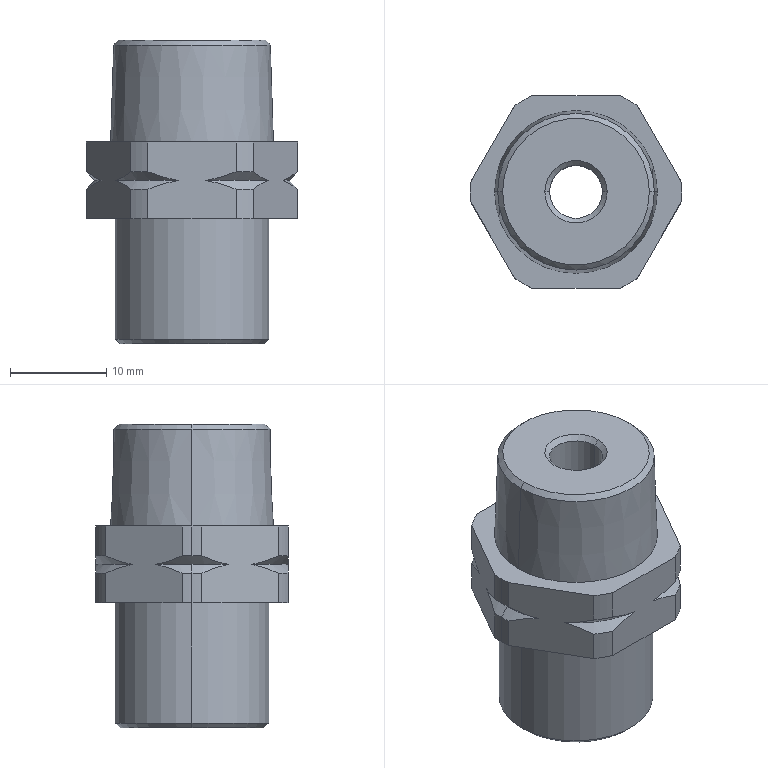Part | STEP file | HXGR200008-06-03-02 | 1 solid | 52 faces | box 22 x 20 x 31.6 mm | volume 6606 mm3 | cone 24 | cylinder 18 | plane 10 | commonest cylinder face diameters 22 x14 5.5 x2 16 x2